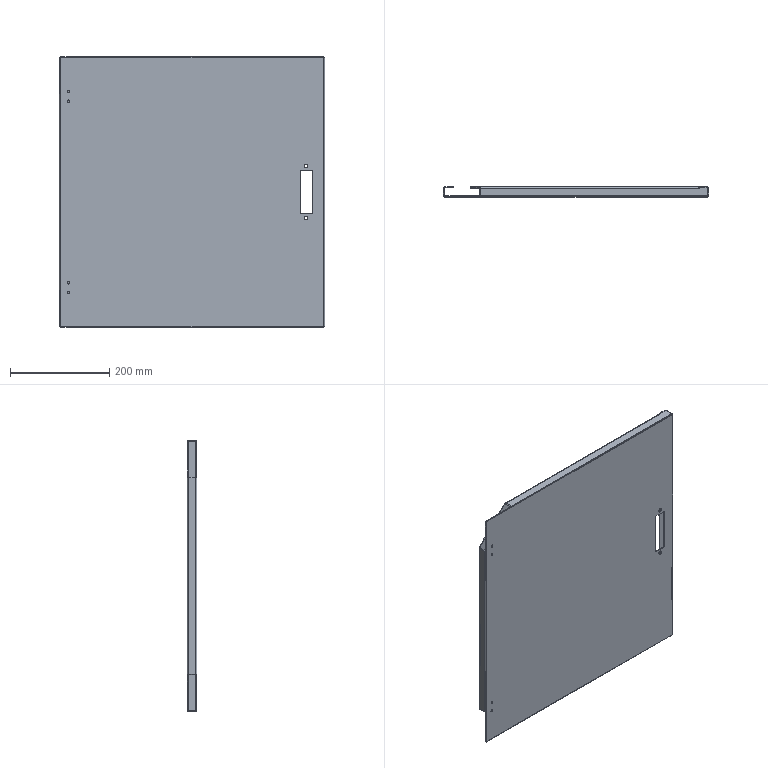Part | NX | features BREP 1 | 1 solid | 82 faces | box 534.5 x 20 x 546 mm | volume 532670 mm3 | plane 56 | cylinder 26 | commonest cylinder face diameters 3 x8 5 x8 6 x6 7.5 x4